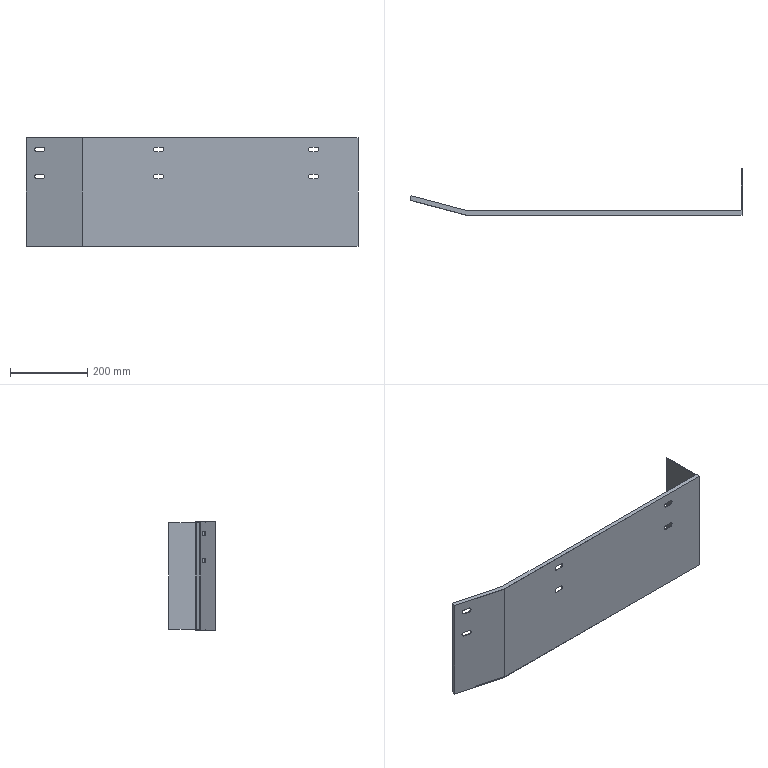Part | SolidWorks | features ICE 3, BossThin 2, LPattern 2, ExtruThin 1 | 1 solid | 48 faces | box 856.99 x 120 x 280 mm | volume 584120 mm3 | plane 30 | cylinder 18 | commonest cylinder face diameters 12 x18
STEP:
#1=CARTESIAN_POINT('',(-808.631,27.69,178.));
#2=VERTEX_POINT('',#1);
#3=CARTESIAN_POINT('',(-814.43,29.228,184.));
#4=VERTEX_POINT('',#3);
#5=CARTESIAN_POINT('',(-814.43,29.228,178.));
#6=DIRECTION('',(-0.2563,-0.9666,0.));
#7=DIRECTION('',(0.9666,-0.2563,0.));
#8=AXIS2_PLACEMENT_3D('',#5,#6,#7);
#9=CIRCLE('',#8,6.);
#10=EDGE_CURVE('',#2,#4,#9,.T.);
#11=ORIENTED_EDGE('',*,*,#10,.F.);
#12=CARTESIAN_POINT('',(-809.143,25.757,178.));
#13=VERTEX_POINT('',#12);
#14=CARTESIAN_POINT('',(-808.631,27.69,178.));
#15=DIRECTION('',(-0.2563,-0.9666,0.));
#16=VECTOR('',#15,1000.);
#17=LINE('',#14,#16);
#18=EDGE_CURVE('',#2,#13,#17,.T.);
#19=ORIENTED_EDGE('',*,*,#18,.T.);
#20=CARTESIAN_POINT('',(-814.943,27.295,184.));
#21=VERTEX_POINT('',#20);
#22=CARTESIAN_POINT('',(-814.943,27.295,178.));
#23=DIRECTION('',(-0.2563,-0.9666,0.));
#24=DIRECTION('',(0.9666,-0.2563,0.));
#25=AXIS2_PLACEMENT_3D('',#22,#23,#24);
#26=CIRCLE('',#25,6.);
#27=EDGE_CURVE('',#13,#21,#26,.T.);
#28=ORIENTED_EDGE('',*,*,#27,.T.);
#29=CARTESIAN_POINT('',(-814.43,29.228,184.));
#30=DIRECTION('',(-0.2563,-0.9666,0.));
#31=VECTOR('',#30,1000.);
#32=LINE('',#29,#31);
#33=EDGE_CURVE('',#4,#21,#32,.T.);
#34=ORIENTED_EDGE('',*,*,#33,.F.);
#35=EDGE_LOOP('',(#11,#19,#28,#34));
#36=FACE_OUTER_BOUND('',#35,.T.);
#37=CARTESIAN_POINT('',(-814.43,29.228,178.));
#38=DIRECTION('',(-0.2563,-0.9666,0.));
#39=DIRECTION('',(0.9666,-0.2563,0.));
#40=AXIS2_PLACEMENT_3D('',#37,#38,#39);
#41=CYLINDRICAL_SURFACE('',#40,6.);
#42=ADVANCED_FACE('',(#36),#41,.F.);
#43=CARTESIAN_POINT('',(-808.631,27.69,248.));
#44=VERTEX_POINT('',#43);
#45=CARTESIAN_POINT('',(-814.43,29.228,254.));
#46=VERTEX_POINT('',#45);
#47=CARTESIAN_POINT('',(-814.43,29.228,248.));
#48=DIRECTION('',(-0.2563,-0.9666,0.));
#49=DIRECTION('',(0.9666,-0.2563,0.));
#50=AXIS2_PLACEMENT_3D('',#47,#48,#49);
#51=CIRCLE('',#50,6.);
#52=EDGE_CURVE('',#44,#46,#51,.T.);
#53=ORIENTED_EDGE('',*,*,#52,.F.);
#54=CARTESIAN_POINT('',(-809.143,25.757,248.));
#55=VERTEX_POINT('',#54);
#56=CARTESIAN_POINT('',(-808.631,27.69,248.));
#57=DIRECTION('',(-0.2563,-0.9666,0.));
#58=VECTOR('',#57,1000.);
#59=LINE('',#56,#58);
#60=EDGE_CURVE('',#44,#55,#59,.T.);
#61=ORIENTED_EDGE('',*,*,#60,.T.);
#62=CARTESIAN_POINT('',(-814.943,27.295,254.));
#63=VERTEX_POINT('',#62);
#64=CARTESIAN_POINT('',(-814.943,27.295,248.));
#65=DIRECTION('',(-0.2563,-0.9666,0.));
#66=DIRECTION('',(0.9666,-0.2563,0.));
#67=AXIS2_PLACEMENT_3D('',#64,#65,#66);
#68=CIRCLE('',#67,6.);
#69=EDGE_CURVE('',#55,#63,#68,.T.);
#70=ORIENTED_EDGE('',*,*,#69,.T.);
#71=CARTESIAN_POINT('',(-814.43,29.228,254.));
#72=DIRECTION('',(-0.2563,-0.9666,0.));
#73=VECTOR('',#72,1000.);
#74=LINE('',#71,#73);
#75=EDGE_CURVE('',#46,#63,#74,.T.);
#76=ORIENTED_EDGE('',*,*,#75,.F.);
#77=EDGE_LOOP('',(#53,#61,#70,#76));
#78=FACE_OUTER_BOUND('',#77,.T.);
#79=CARTESIAN_POINT('',(-814.43,29.228,248.));
#80=DIRECTION('',(-0.2563,-0.9666,0.));
#81=DIRECTION('',(0.9666,-0.2563,0.));
#82=AXIS2_PLACEMENT_3D('',#79,#80,#81);
#83=CYLINDRICAL_SURFACE('',#82,6.);
#84=ADVANCED_FACE('',(#78),#83,.F.);
#85=CARTESIAN_POINT('',(-501.5,2.,178.));
#86=VERTEX_POINT('',#85);
#87=CARTESIAN_POINT('',(-507.5,2.,184.));
#88=VERTEX_POINT('',#87);
#89=CARTESIAN_POINT('',(-507.5,2.,178.));
#90=DIRECTION('',(0.,-1.,0.));
#91=DIRECTION('',(1.,0.,0.));
#92=AXIS2_PLACEMENT_3D('',#89,#90,#91);
#93=CIRCLE('',#92,6.);
#94=EDGE_CURVE('',#86,#88,#93,.T.);
#95=ORIENTED_EDGE('',*,*,#94,.F.);
#96=CARTESIAN_POINT('',(-501.5,0.,178.));
#97=VERTEX_POINT('',#96);
#98=CARTESIAN_POINT('',(-501.5,2.,178.));
#99=DIRECTION('',(0.,-1.,0.));
#100=VECTOR('',#99,1000.);
#101=LINE('',#98,#100);
#102=EDGE_CURVE('',#86,#97,#101,.T.);
#103=ORIENTED_EDGE('',*,*,#102,.T.);
#104=CARTESIAN_POINT('',(-507.5,0.,184.));
#105=VERTEX_POINT('',#104);
#106=CARTESIAN_POINT('',(-507.5,0.,178.));
#107=DIRECTION('',(0.,-1.,0.));
#108=DIRECTION('',(1.,0.,0.));
#109=AXIS2_PLACEMENT_3D('',#106,#107,#108);
#110=CIRCLE('',#109,6.);
#111=EDGE_CURVE('',#97,#105,#110,.T.);
#112=ORIENTED_EDGE('',*,*,#111,.T.);
#113=CARTESIAN_POINT('',(-507.5,2.,184.));
#114=DIRECTION('',(0.,-1.,0.));
#115=VECTOR('',#114,1000.);
#116=LINE('',#113,#115);
#117=EDGE_CURVE('',#88,#105,#116,.T.);
#118=ORIENTED_EDGE('',*,*,#117,.F.);
#119=EDGE_LOOP('',(#95,#103,#112,#118));
#120=FACE_OUTER_BOUND('',#119,.T.);
#121=CARTESIAN_POINT('',(-507.5,2.,178.));
#122=DIRECTION('',(0.,-1.,0.));
#123=DIRECTION('',(1.,0.,0.));
#124=AXIS2_PLACEMENT_3D('',#121,#122,#123);
#125=CYLINDRICAL_SURFACE('',#124,6.);
#126=ADVANCED_FACE('',(#120),#125,.F.);
#127=CARTESIAN_POINT('',(-101.5,2.,178.));
#128=VERTEX_POINT('',#127);
#129=CARTESIAN_POINT('',(-107.5,2.,184.));
#130=VERTEX_POINT('',#129);
#131=CARTESIAN_POINT('',(-107.5,2.,178.));
#132=DIRECTION('',(0.,-1.,0.));
#133=DIRECTION('',(1.,0.,0.));
#134=AXIS2_PLACEMENT_3D('',#131,#132,#133);
#135=CIRCLE('',#134,6.);
#136=EDGE_CURVE('',#128,#130,#135,.T.);
#137=ORIENTED_EDGE('',*,*,#136,.F.);
#138=CARTESIAN_POINT('',(-101.5,0.,178.));
#139=VERTEX_POINT('',#138);
#140=CARTESIAN_POINT('',(-101.5,2.,178.));
#141=DIRECTION('',(0.,-1.,0.));
#142=VECTOR('',#141,1000.);
#143=LINE('',#140,#142);
#144=EDGE_CURVE('',#128,#139,#143,.T.);
#145=ORIENTED_EDGE('',*,*,#144,.T.);
#146=CARTESIAN_POINT('',(-107.5,0.,184.));
#147=VERTEX_POINT('',#146);
#148=CARTESIAN_POINT('',(-107.5,0.,178.));
#149=DIRECTION('',(0.,-1.,0.));
#150=DIRECTION('',(1.,0.,0.));
#151=AXIS2_PLACEMENT_3D('',#148,#149,#150);
#152=CIRCLE('',#151,6.);
#153=EDGE_CURVE('',#139,#147,#152,.T.);
#154=ORIENTED_EDGE('',*,*,#153,.T.);
#155=CARTESIAN_POINT('',(-107.5,2.,184.));
#156=DIRECTION('',(0.,-1.,0.));
#157=VECTOR('',#156,1000.);
#158=LINE('',#155,#157);
#159=EDGE_CURVE('',#130,#147,#158,.T.);
#160=ORIENTED_EDGE('',*,*,#159,.F.);
#161=EDGE_LOOP('',(#137,#145,#154,#160));
#162=FACE_OUTER_BOUND('',#161,.T.);
#163=CARTESIAN_POINT('',(-107.5,2.,178.));
#164=DIRECTION('',(0.,-1.,0.));
#165=DIRECTION('',(1.,0.,0.));
#166=AXIS2_PLACEMENT_3D('',#163,#164,#165);
#167=CYLINDRICAL_SURFACE('',#166,6.);
#168=ADVANCED_FACE('',(#162),#167,.F.);
#169=CARTESIAN_POINT('',(-501.5,2.,248.));
#170=VERTEX_POINT('',#169);
#171=CARTESIAN_POINT('',(-507.5,2.,254.));
#172=VERTEX_POINT('',#171);
#173=CARTESIAN_POINT('',(-507.5,2.,248.));
#174=DIRECTION('',(0.,-1.,0.));
#175=DIRECTION('',(1.,0.,0.));
#176=AXIS2_PLACEMENT_3D('',#173,#174,#175);
#177=CIRCLE('',#176,6.);
#178=EDGE_CURVE('',#170,#172,#177,.T.);
#179=ORIENTED_EDGE('',*,*,#178,.F.);
#180=CARTESIAN_POINT('',(-501.5,0.,248.));
#181=VERTEX_POINT('',#180);
#182=CARTESIAN_POINT('',(-501.5,2.,248.));
#183=DIRECTION('',(0.,-1.,0.));
#184=VECTOR('',#183,1000.);
#185=LINE('',#182,#184);
#186=EDGE_CURVE('',#170,#181,#185,.T.);
#187=ORIENTED_EDGE('',*,*,#186,.T.);
#188=CARTESIAN_POINT('',(-507.5,0.,254.));
#189=VERTEX_POINT('',#188);
#190=CARTESIAN_POINT('',(-507.5,0.,248.));
#191=DIRECTION('',(0.,-1.,0.));
#192=DIRECTION('',(1.,0.,0.));
#193=AXIS2_PLACEMENT_3D('',#190,#191,#192);
#194=CIRCLE('',#193,6.);
#195=EDGE_CURVE('',#181,#189,#194,.T.);
#196=ORIENTED_EDGE('',*,*,#195,.T.);
#197=CARTESIAN_POINT('',(-507.5,2.,254.));
#198=DIRECTION('',(0.,-1.,0.));
#199=VECTOR('',#198,1000.);
#200=LINE('',#197,#199);
#201=EDGE_CURVE('',#172,#189,#200,.T.);
#202=ORIENTED_EDGE('',*,*,#201,.F.);
#203=EDGE_LOOP('',(#179,#187,#196,#202));
#204=FACE_OUTER_BOUND('',#203,.T.);
#205=CARTESIAN_POINT('',(-507.5,2.,248.));
#206=DIRECTION('',(0.,-1.,0.));
#207=DIRECTION('',(1.,0.,0.));
#208=AXIS2_PLACEMENT_3D('',#205,#206,#207);
#209=CYLINDRICAL_SURFACE('',#208,6.);
#210=ADVANCED_FACE('',(#204),#209,.F.);
#211=CARTESIAN_POINT('',(-101.5,2.,248.));
#212=VERTEX_POINT('',#211);
#213=CARTESIAN_POINT('',(-107.5,2.,254.));
#214=VERTEX_POINT('',#213);
#215=CARTESIAN_POINT('',(-107.5,2.,248.));
#216=DIRECTION('',(0.,-1.,0.));
#217=DIRECTION('',(1.,0.,0.));
#218=AXIS2_PLACEMENT_3D('',#215,#216,#217);
#219=CIRCLE('',#218,6.);
#220=EDGE_CURVE('',#212,#214,#219,.T.);
#221=ORIENTED_EDGE('',*,*,#220,.F.);
#222=CARTESIAN_POINT('',(-101.5,0.,248.));
#223=VERTEX_POINT('',#222);
#224=CARTESIAN_POINT('',(-101.5,2.,248.));
#225=DIRECTION('',(0.,-1.,0.));
#226=VECTOR('',#225,1000.);
#227=LINE('',#224,#226);
#228=EDGE_CURVE('',#212,#223,#227,.T.);
#229=ORIENTED_EDGE('',*,*,#228,.T.);
#230=CARTESIAN_POINT('',(-107.5,0.,254.));
#231=VERTEX_POINT('',#230);
#232=CARTESIAN_POINT('',(-107.5,0.,248.));
#233=DIRECTION('',(0.,-1.,0.));
#234=DIRECTION('',(1.,0.,0.));
#235=AXIS2_PLACEMENT_3D('',#232,#233,#234);
#236=CIRCLE('',#235,6.);
#237=EDGE_CURVE('',#223,#231,#236,.T.);
#238=ORIENTED_EDGE('',*,*,#237,.T.);
#239=CARTESIAN_POINT('',(-107.5,2.,254.));
#240=DIRECTION('',(0.,-1.,0.));
#241=VECTOR('',#240,1000.);
#242=LINE('',#239,#241);
#243=EDGE_CURVE('',#214,#231,#242,.T.);
#244=ORIENTED_EDGE('',*,*,#243,.F.);
#245=EDGE_LOOP('',(#221,#229,#238,#244));
#246=FACE_OUTER_BOUND('',#245,.T.);
#247=CARTESIAN_POINT('',(-107.5,2.,248.));
#248=DIRECTION('',(0.,-1.,0.));
#249=DIRECTION('',(1.,0.,0.));
#250=AXIS2_PLACEMENT_3D('',#247,#248,#249);
#251=CYLINDRICAL_SURFACE('',#250,6.);
#252=ADVANCED_FACE('',(#246),#251,.F.);
#253=CARTESIAN_POINT('',(-828.929,33.072,254.));
#254=VERTEX_POINT('',#253);
#255=CARTESIAN_POINT('',(-828.929,33.072,254.));
#256=DIRECTION('',(-0.9666,0.2563,0.));
#257=VECTOR('',#256,1000.);
#258=LINE('',#255,#257);
#259=EDGE_CURVE('',#46,#254,#258,.T.);
#260=ORIENTED_EDGE('',*,*,#259,.T.);
#261=CARTESIAN_POINT('',(-828.929,33.072,242.));
#262=VERTEX_POINT('',#261);
#263=CARTESIAN_POINT('',(-828.929,33.072,248.));
#264=DIRECTION('',(-0.2563,-0.9666,0.));
#265=DIRECTION('',(0.9666,-0.2563,0.));
#266=AXIS2_PLACEMENT_3D('',#263,#264,#265);
#267=CIRCLE('',#266,6.);
#268=EDGE_CURVE('',#254,#262,#267,.T.);
#269=ORIENTED_EDGE('',*,*,#268,.T.);
#270=CARTESIAN_POINT('',(-814.43,29.228,242.));
#271=VERTEX_POINT('',#270);
#272=CARTESIAN_POINT('',(-828.929,33.072,242.));
#273=DIRECTION('',(0.9666,-0.2563,0.));
#274=VECTOR('',#273,1000.);
#275=LINE('',#272,#274);
#276=EDGE_CURVE('',#262,#271,#275,.T.);
#277=ORIENTED_EDGE('',*,*,#276,.T.);
#278=CARTESIAN_POINT('',(-814.43,29.228,248.));
#279=DIRECTION('',(-0.2563,-0.9666,0.));
#280=DIRECTION('',(0.9666,-0.2563,0.));
#281=AXIS2_PLACEMENT_3D('',#278,#279,#280);
#282=CIRCLE('',#281,6.);
#283=EDGE_CURVE('',#271,#44,#282,.T.);
#284=ORIENTED_EDGE('',*,*,#283,.T.);
#285=ORIENTED_EDGE('',*,*,#52,.T.);
#286=EDGE_LOOP('',(#260,#269,#277,#284,#285));
#287=FACE_BOUND('',#286,.T.);
#288=CARTESIAN_POINT('',(-828.929,33.072,184.));
#289=VERTEX_POINT('',#288);
#290=CARTESIAN_POINT('',(-828.929,33.072,184.));
#291=DIRECTION('',(-0.9666,0.2563,0.));
#292=VECTOR('',#291,1000.);
#293=LINE('',#290,#292);
#294=EDGE_CURVE('',#4,#289,#293,.T.);
#295=ORIENTED_EDGE('',*,*,#294,.T.);
#296=CARTESIAN_POINT('',(-828.929,33.072,172.));
#297=VERTEX_POINT('',#296);
#298=CARTESIAN_POINT('',(-828.929,33.072,178.));
#299=DIRECTION('',(-0.2563,-0.9666,0.));
#300=DIRECTION('',(0.9666,-0.2563,0.));
#301=AXIS2_PLACEMENT_3D('',#298,#299,#300);
#302=CIRCLE('',#301,6.);
#303=EDGE_CURVE('',#289,#297,#302,.T.);
#304=ORIENTED_EDGE('',*,*,#303,.T.);
#305=CARTESIAN_POINT('',(-814.43,29.228,172.));
#306=VERTEX_POINT('',#305);
#307=CARTESIAN_POINT('',(-828.929,33.072,172.));
#308=DIRECTION('',(0.9666,-0.2563,0.));
#309=VECTOR('',#308,1000.);
#310=LINE('',#307,#309);
#311=EDGE_CURVE('',#297,#306,#310,.T.);
#312=ORIENTED_EDGE('',*,*,#311,.T.);
#313=CARTESIAN_POINT('',(-814.43,29.228,178.));
#314=DIRECTION('',(-0.2563,-0.9666,0.));
#315=DIRECTION('',(0.9666,-0.2563,0.));
#316=AXIS2_PLACEMENT_3D('',#313,#314,#315);
#317=CIRCLE('',#316,6.);
#318=EDGE_CURVE('',#306,#2,#317,.T.);
#319=ORIENTED_EDGE('',*,*,#318,.T.);
#320=ORIENTED_EDGE('',*,*,#10,.T.);
#321=EDGE_LOOP('',(#295,#304,#312,#319,#320));
#322=FACE_BOUND('',#321,.T.);
#323=CARTESIAN_POINT('',(-854.544,39.864,276.));
#324=VERTEX_POINT('',#323);
#325=CARTESIAN_POINT('',(-854.544,39.864,0.));
#326=VERTEX_POINT('',#325);
#327=CARTESIAN_POINT('',(-854.544,39.864,0.));
#328=DIRECTION('',(0.,0.,-1.));
#329=VECTOR('',#328,1000.);
#330=LINE('',#327,#329);
#331=EDGE_CURVE('',#324,#326,#330,.T.);
#332=ORIENTED_EDGE('',*,*,#331,.F.);
#333=CARTESIAN_POINT('',(-711.739,2.,276.));
#334=VERTEX_POINT('',#333);
#335=CARTESIAN_POINT('',(-711.487,1.933,276.));
#336=DIRECTION('',(-0.9666,0.2563,0.));
#337=VECTOR('',#336,1000.);
#338=LINE('',#335,#337);
#339=EDGE_CURVE('',#334,#324,#338,.T.);
#340=ORIENTED_EDGE('',*,*,#339,.F.);
#341=CARTESIAN_POINT('',(-711.739,2.,0.));
#342=VERTEX_POINT('',#341);
#343=CARTESIAN_POINT('',(-711.739,2.,276.));
#344=DIRECTION('',(0.,0.,-1.));
#345=VECTOR('',#344,1000.);
#346=LINE('',#343,#345);
#347=EDGE_CURVE('',#334,#342,#346,.T.);
#348=ORIENTED_EDGE('',*,*,#347,.T.);
#349=CARTESIAN_POINT('',(-711.487,1.933,0.));
#350=DIRECTION('',(-0.9666,0.2563,0.));
#351=VECTOR('',#350,1000.);
#352=LINE('',#349,#351);
#353=EDGE_CURVE('',#342,#326,#352,.T.);
#354=ORIENTED_EDGE('',*,*,#353,.T.);
#355=EDGE_LOOP('',(#332,#340,#348,#354));
#356=FACE_OUTER_BOUND('',#355,.T.);
#357=CARTESIAN_POINT('',(-711.487,1.933,276.));
#358=DIRECTION('',(-0.2563,-0.9666,0.));
#359=DIRECTION('',(0.9666,-0.2563,0.));
#360=AXIS2_PLACEMENT_3D('',#357,#358,#359);
#361=PLANE('',#360);
#362=ADVANCED_FACE('',(#287,#322,#356),#361,.F.);
#363=ORIENTED_EDGE('',*,*,#339,.T.);
#364=CARTESIAN_POINT('',(-851.981,49.53,276.));
#365=VERTEX_POINT('',#364);
#366=CARTESIAN_POINT('',(-851.981,49.53,276.));
#367=DIRECTION('',(-0.2563,-0.9666,0.));
#368=VECTOR('',#367,1000.);
#369=LINE('',#366,#368);
#370=EDGE_CURVE('',#365,#324,#369,.T.);
#371=ORIENTED_EDGE('',*,*,#370,.F.);
#372=CARTESIAN_POINT('',(-710.436,12.,276.));
#373=VERTEX_POINT('',#372);
#374=CARTESIAN_POINT('',(-708.925,11.599,276.));
#375=DIRECTION('',(-0.9666,0.2563,0.));
#376=VECTOR('',#375,1000.);
#377=LINE('',#374,#376);
#378=EDGE_CURVE('',#373,#365,#377,.T.);
#379=ORIENTED_EDGE('',*,*,#378,.F.);
#380=CARTESIAN_POINT('',(-2.,12.,276.));
#381=VERTEX_POINT('',#380);
#382=CARTESIAN_POINT('',(0.,12.,276.));
#383=DIRECTION('',(-1.,0.,0.));
#384=VECTOR('',#383,1000.);
#385=LINE('',#382,#384);
#386=EDGE_CURVE('',#381,#373,#385,.T.);
#387=ORIENTED_EDGE('',*,*,#386,.F.);
#388=CARTESIAN_POINT('',(-2.,2.,276.));
#389=VERTEX_POINT('',#388);
#390=CARTESIAN_POINT('',(-2.,0.,276.));
#391=DIRECTION('',(0.,-1.,0.));
#392=VECTOR('',#391,1000.);
#393=LINE('',#390,#392);
#394=EDGE_CURVE('',#381,#389,#393,.T.);
#395=ORIENTED_EDGE('',*,*,#394,.T.);
#396=CARTESIAN_POINT('',(0.,2.,276.));
#397=DIRECTION('',(-1.,0.,0.));
#398=VECTOR('',#397,1000.);
#399=LINE('',#396,#398);
#400=EDGE_CURVE('',#389,#334,#399,.T.);
#401=ORIENTED_EDGE('',*,*,#400,.T.);
#402=EDGE_LOOP('',(#363,#371,#379,#387,#395,#401));
#403=FACE_OUTER_BOUND('',#402,.T.);
#404=CARTESIAN_POINT('',(0.,0.,276.));
#405=DIRECTION('',(0.,0.,-1.));
#406=DIRECTION('',(-1.,0.,0.));
#407=AXIS2_PLACEMENT_3D('',#404,#405,#406);
#408=PLANE('',#407);
#409=ADVANCED_FACE('',(#403),#408,.T.);
#410=CARTESIAN_POINT('',(-710.436,12.,0.));
#411=VERTEX_POINT('',#410);
#412=CARTESIAN_POINT('',(-851.981,49.53,0.));
#413=VERTEX_POINT('',#412);
#414=CARTESIAN_POINT('',(-708.925,11.599,0.));
#415=DIRECTION('',(-0.9666,0.2563,0.));
#416=VECTOR('',#415,1000.);
#417=LINE('',#414,#416);
#418=EDGE_CURVE('',#411,#413,#417,.T.);
#419=ORIENTED_EDGE('',*,*,#418,.T.);
#420=CARTESIAN_POINT('',(-851.981,49.53,0.));
#421=DIRECTION('',(-0.2563,-0.9666,0.));
#422=VECTOR('',#421,1000.);
#423=LINE('',#420,#422);
#424=EDGE_CURVE('',#413,#326,#423,.T.);
#425=ORIENTED_EDGE('',*,*,#424,.T.);
#426=ORIENTED_EDGE('',*,*,#353,.F.);
#427=CARTESIAN_POINT('',(-2.,2.,0.));
#428=VERTEX_POINT('',#427);
#429=CARTESIAN_POINT('',(0.,2.,0.));
#430=DIRECTION('',(-1.,0.,0.));
#431=VECTOR('',#430,1000.);
#432=LINE('',#429,#431);
#433=EDGE_CURVE('',#428,#342,#432,.T.);
#434=ORIENTED_EDGE('',*,*,#433,.F.);
#435=CARTESIAN_POINT('',(-2.,12.,0.));
#436=VERTEX_POINT('',#435);
#437=CARTESIAN_POINT('',(-2.,0.,0.));
#438=DIRECTION('',(0.,-1.,0.));
#439=VECTOR('',#438,1000.);
#440=LINE('',#437,#439);
#441=EDGE_CURVE('',#436,#428,#440,.T.);
#442=ORIENTED_EDGE('',*,*,#441,.F.);
#443=CARTESIAN_POINT('',(0.,12.,0.));
#444=DIRECTION('',(-1.,0.,0.));
#445=VECTOR('',#444,1000.);
#446=LINE('',#443,#445);
#447=EDGE_CURVE('',#436,#411,#446,.T.);
#448=ORIENTED_EDGE('',*,*,#447,.T.);
#449=EDGE_LOOP('',(#419,#425,#426,#434,#442,#448));
#450=FACE_OUTER_BOUND('',#449,.T.);
#451=CARTESIAN_POINT('',(0.,0.,0.));
#452=DIRECTION('',(0.,0.,1.));
#453=DIRECTION('',(1.,0.,0.));
#454=AXIS2_PLACEMENT_3D('',#451,#452,#453);
#455=PLANE('',#454);
#456=ADVANCED_FACE('',(#450),#455,.T.);
#457=CARTESIAN_POINT('',(0.,120.,0.));
#458=VERTEX_POINT('',#457);
#459=CARTESIAN_POINT('',(0.,12.,0.));
#460=VERTEX_POINT('',#459);
#461=CARTESIAN_POINT('',(0.,0.,0.));
#462=DIRECTION('',(0.,-1.,0.));
#463=VECTOR('',#462,1000.);
#464=LINE('',#461,#463);
#465=EDGE_CURVE('',#458,#460,#464,.T.);
#466=ORIENTED_EDGE('',*,*,#465,.T.);
#467=CARTESIAN_POINT('',(0.,12.,0.));
#468=DIRECTION('',(-1.,0.,0.));
#469=VECTOR('',#468,1000.);
#470=LINE('',#467,#469);
#471=EDGE_CURVE('',#460,#436,#470,.T.);
#472=ORIENTED_EDGE('',*,*,#471,.T.);
#473=CARTESIAN_POINT('',(-2.,120.,0.));
#474=VERTEX_POINT('',#473);
#475=CARTESIAN_POINT('',(-2.,0.,0.));
#476=DIRECTION('',(0.,-1.,0.));
#477=VECTOR('',#476,1000.);
#478=LINE('',#475,#477);
#479=EDGE_CURVE('',#474,#436,#478,.T.);
#480=ORIENTED_EDGE('',*,*,#479,.F.);
#481=CARTESIAN_POINT('',(-2.,120.,0.));
#482=DIRECTION('',(1.,0.,0.));
#483=VECTOR('',#482,1000.);
#484=LINE('',#481,#483);
#485=EDGE_CURVE('',#474,#458,#484,.T.);
#486=ORIENTED_EDGE('',*,*,#485,.T.);
#487=EDGE_LOOP('',(#466,#472,#480,#486));
#488=FACE_OUTER_BOUND('',#487,.T.);
#489=CARTESIAN_POINT('',(0.,0.,0.));
#490=DIRECTION('',(0.,0.,-1.));
#491=DIRECTION('',(-1.,0.,0.));
#492=AXIS2_PLACEMENT_3D('',#489,#490,#491);
#493=PLANE('',#492);
#494=ADVANCED_FACE('',(#488),#493,.T.);
#495=CARTESIAN_POINT('',(0.,12.,276.));
#496=VERTEX_POINT('',#495);
#497=CARTESIAN_POINT('',(0.,12.,276.));
#498=DIRECTION('',(-1.,0.,0.));
#499=VECTOR('',#498,1000.);
#500=LINE('',#497,#499);
#501=EDGE_CURVE('',#496,#381,#500,.T.);
#502=ORIENTED_EDGE('',*,*,#501,.F.);
#503=CARTESIAN_POINT('',(0.,120.,276.));
#504=VERTEX_POINT('',#503);
#505=CARTESIAN_POINT('',(0.,0.,276.));
#506=DIRECTION('',(0.,-1.,0.));
#507=VECTOR('',#506,1000.);
#508=LINE('',#505,#507);
#509=EDGE_CURVE('',#504,#496,#508,.T.);
#510=ORIENTED_EDGE('',*,*,#509,.F.);
#511=CARTESIAN_POINT('',(-2.,120.,276.));
#512=VERTEX_POINT('',#511);
#513=CARTESIAN_POINT('',(-2.,120.,276.));
#514=DIRECTION('',(1.,0.,0.));
#515=VECTOR('',#514,1000.);
#516=LINE('',#513,#515);
#517=EDGE_CURVE('',#512,#504,#516,.T.);
#518=ORIENTED_EDGE('',*,*,#517,.F.);
#519=CARTESIAN_POINT('',(-2.,0.,276.));
#520=DIRECTION('',(0.,-1.,0.));
#521=VECTOR('',#520,1000.);
#522=LINE('',#519,#521);
#523=EDGE_CURVE('',#512,#381,#522,.T.);
#524=ORIENTED_EDGE('',*,*,#523,.T.);
#525=EDGE_LOOP('',(#502,#510,#518,#524));
#526=FACE_OUTER_BOUND('',#525,.T.);
#527=CARTESIAN_POINT('',(0.,0.,276.));
#528=DIRECTION('',(0.,0.,-1.));
#529=DIRECTION('',(-1.,0.,0.));
#530=AXIS2_PLACEMENT_3D('',#527,#528,#529);
#531=PLANE('',#530);
#532=ADVANCED_FACE('',(#526),#531,.F.);
#533=CARTESIAN_POINT('',(-853.915,50.043,278.));
#534=VERTEX_POINT('',#533);
#535=CARTESIAN_POINT('',(-853.915,50.043,-2.));
#536=VERTEX_POINT('',#535);
#537=CARTESIAN_POINT('',(-853.915,50.043,278.));
#538=DIRECTION('',(0.,0.,-1.));
#539=VECTOR('',#538,1000.);
#540=LINE('',#537,#539);
#541=EDGE_CURVE('',#534,#536,#540,.T.);
#542=ORIENTED_EDGE('',*,*,#541,.T.);
#543=CARTESIAN_POINT('',(-856.99,38.443,-2.));
#544=VERTEX_POINT('',#543);
#545=CARTESIAN_POINT('',(-853.915,50.043,-2.));
#546=DIRECTION('',(-0.2563,-0.9666,0.));
#547=VECTOR('',#546,1000.);
#548=LINE('',#545,#547);
#549=EDGE_CURVE('',#536,#544,#548,.T.);
#550=ORIENTED_EDGE('',*,*,#549,.T.);
#551=CARTESIAN_POINT('',(-856.99,38.443,278.));
#552=VERTEX_POINT('',#551);
#553=CARTESIAN_POINT('',(-856.99,38.443,276.));
#554=DIRECTION('',(0.,0.,-1.));
#555=VECTOR('',#554,1000.);
#556=LINE('',#553,#555);
#557=EDGE_CURVE('',#552,#544,#556,.T.);
#558=ORIENTED_EDGE('',*,*,#557,.F.);
#559=CARTESIAN_POINT('',(-856.99,38.443,278.));
#560=DIRECTION('',(0.2563,0.9666,0.));
#561=VECTOR('',#560,1000.);
#562=LINE('',#559,#561);
#563=EDGE_CURVE('',#552,#534,#562,.T.);
#564=ORIENTED_EDGE('',*,*,#563,.T.);
#565=EDGE_LOOP('',(#542,#550,#558,#564));
#566=FACE_OUTER_BOUND('',#565,.T.);
#567=CARTESIAN_POINT('',(-856.99,38.443,276.));
#568=DIRECTION('',(-0.9666,0.2563,0.));
#569=DIRECTION('',(-0.2563,-0.9666,0.));
#570=AXIS2_PLACEMENT_3D('',#567,#568,#569);
#571=PLANE('',#570);
#572=ADVANCED_FACE('',(#566),#571,.T.);
#573=CARTESIAN_POINT('',(-829.442,31.139,184.));
#574=VERTEX_POINT('',#573);
#575=CARTESIAN_POINT('',(-829.442,31.139,172.));
#576=VERTEX_POINT('',#575);
#577=CARTESIAN_POINT('',(-829.442,31.139,178.));
#578=DIRECTION('',(-0.2563,-0.9666,0.));
#579=DIRECTION('',(0.9666,-0.2563,0.));
#580=AXIS2_PLACEMENT_3D('',#577,#578,#579);
#581=CIRCLE('',#580,6.);
#582=EDGE_CURVE('',#574,#576,#581,.T.);
#583=ORIENTED_EDGE('',*,*,#582,.F.);
#584=CARTESIAN_POINT('',(-829.442,31.139,184.));
#585=DIRECTION('',(-0.9666,0.2563,0.));
#586=VECTOR('',#585,1000.);
#587=LINE('',#584,#586);
#588=EDGE_CURVE('',#21,#574,#587,.T.);
#589=ORIENTED_EDGE('',*,*,#588,.F.);
#590=ORIENTED_EDGE('',*,*,#27,.F.);
#591=CARTESIAN_POINT('',(-814.943,27.295,172.));
#592=VERTEX_POINT('',#591);
#593=CARTESIAN_POINT('',(-814.943,27.295,178.));
#594=DIRECTION('',(-0.2563,-0.9666,0.));
#595=DIRECTION('',(0.9666,-0.2563,0.));
#596=AXIS2_PLACEMENT_3D('',#593,#594,#595);
#597=CIRCLE('',#596,6.);
#598=EDGE_CURVE('',#592,#13,#597,.T.);
#599=ORIENTED_EDGE('',*,*,#598,.F.);
#600=CARTESIAN_POINT('',(-829.442,31.139,172.));
#601=DIRECTION('',(0.9666,-0.2563,0.));
#602=VECTOR('',#601,1000.);
#603=LINE('',#600,#602);
#604=EDGE_CURVE('',#576,#592,#603,.T.);
#605=ORIENTED_EDGE('',*,*,#604,.F.);
#606=EDGE_LOOP('',(#583,#589,#590,#599,#605));
#607=FACE_BOUND('',#606,.T.);
#608=CARTESIAN_POINT('',(-829.442,31.139,254.));
#609=VERTEX_POINT('',#608);
#610=CARTESIAN_POINT('',(-829.442,31.139,242.));
#611=VERTEX_POINT('',#610);
#612=CARTESIAN_POINT('',(-829.442,31.139,248.));
#613=DIRECTION('',(-0.2563,-0.9666,0.));
#614=DIRECTION('',(0.9666,-0.2563,0.));
#615=AXIS2_PLACEMENT_3D('',#612,#613,#614);
#616=CIRCLE('',#615,6.);
#617=EDGE_CURVE('',#609,#611,#616,.T.);
#618=ORIENTED_EDGE('',*,*,#617,.F.);
#619=CARTESIAN_POINT('',(-829.442,31.139,254.));
#620=DIRECTION('',(-0.9666,0.2563,0.));
#621=VECTOR('',#620,1000.);
#622=LINE('',#619,#621);
#623=EDGE_CURVE('',#63,#609,#622,.T.);
#624=ORIENTED_EDGE('',*,*,#623,.F.);
#625=ORIENTED_EDGE('',*,*,#69,.F.);
#626=CARTESIAN_POINT('',(-814.943,27.295,242.));
#627=VERTEX_POINT('',#626);
#628=CARTESIAN_POINT('',(-814.943,27.295,248.));
#629=DIRECTION('',(-0.2563,-0.9666,0.));
#630=DIRECTION('',(0.9666,-0.2563,0.));
#631=AXIS2_PLACEMENT_3D('',#628,#629,#630);
#632=CIRCLE('',#631,6.);
#633=EDGE_CURVE('',#627,#55,#632,.T.);
#634=ORIENTED_EDGE('',*,*,#633,.F.);
#635=CARTESIAN_POINT('',(-829.442,31.139,242.));
#636=DIRECTION('',(0.9666,-0.2563,0.));
#637=VECTOR('',#636,1000.);
#638=LINE('',#635,#637);
#639=EDGE_CURVE('',#611,#627,#638,.T.);
#640=ORIENTED_EDGE('',*,*,#639,.F.);
#641=EDGE_LOOP('',(#618,#624,#625,#634,#640));
#642=FACE_BOUND('',#641,.T.);
#643=ORIENTED_EDGE('',*,*,#557,.T.);
#644=CARTESIAN_POINT('',(-712.,0.,-2.));
#645=VERTEX_POINT('',#644);
#646=CARTESIAN_POINT('',(-712.,0.,-2.));
#647=DIRECTION('',(-0.9666,0.2563,0.));
#648=VECTOR('',#647,1000.);
#649=LINE('',#646,#648);
#650=EDGE_CURVE('',#645,#544,#649,.T.);
#651=ORIENTED_EDGE('',*,*,#650,.F.);
#652=CARTESIAN_POINT('',(-712.,0.,278.));
#653=VERTEX_POINT('',#652);
#654=CARTESIAN_POINT('',(-712.,0.,276.));
#655=DIRECTION('',(0.,0.,-1.));
#656=VECTOR('',#655,1000.);
#657=LINE('',#654,#656);
#658=EDGE_CURVE('',#653,#645,#657,.T.);
#659=ORIENTED_EDGE('',*,*,#658,.F.);
#660=CARTESIAN_POINT('',(-712.,0.,278.));
#661=DIRECTION('',(-0.9666,0.2563,0.));
#662=VECTOR('',#661,1000.);
#663=LINE('',#660,#662);
#664=EDGE_CURVE('',#653,#552,#663,.T.);
#665=ORIENTED_EDGE('',*,*,#664,.T.);
#666=EDGE_LOOP('',(#643,#651,#659,#665));
#667=FACE_OUTER_BOUND('',#666,.T.);
#668=CARTESIAN_POINT('',(-712.,0.,276.));
#669=DIRECTION('',(-0.2563,-0.9666,0.));
#670=DIRECTION('',(0.9666,-0.2563,0.));
#671=AXIS2_PLACEMENT_3D('',#668,#669,#670);
#672=PLANE('',#671);
#673=ADVANCED_FACE('',(#607,#642,#667),#672,.T.);
#674=CARTESIAN_POINT('',(-522.5,0.,254.));
#675=VERTEX_POINT('',#674);
#676=CARTESIAN_POINT('',(-522.5,0.,242.));
#677=VERTEX_POINT('',#676);
#678=CARTESIAN_POINT('',(-522.5,0.,248.));
#679=DIRECTION('',(0.,-1.,0.));
#680=DIRECTION('',(1.,0.,0.));
#681=AXIS2_PLACEMENT_3D('',#678,#679,#680);
#682=CIRCLE('',#681,6.);
#683=EDGE_CURVE('',#675,#677,#682,.T.);
#684=ORIENTED_EDGE('',*,*,#683,.F.);
#685=CARTESIAN_POINT('',(-522.5,0.,254.));
#686=DIRECTION('',(-1.,0.,0.));
#687=VECTOR('',#686,1000.);
#688=LINE('',#685,#687);
#689=EDGE_CURVE('',#189,#675,#688,.T.);
#690=ORIENTED_EDGE('',*,*,#689,.F.);
#691=ORIENTED_EDGE('',*,*,#195,.F.);
#692=CARTESIAN_POINT('',(-507.5,0.,242.));
#693=VERTEX_POINT('',#692);
#694=CARTESIAN_POINT('',(-507.5,0.,248.));
#695=DIRECTION('',(0.,-1.,0.));
#696=DIRECTION('',(1.,0.,0.));
#697=AXIS2_PLACEMENT_3D('',#694,#695,#696);
#698=CIRCLE('',#697,6.);
#699=EDGE_CURVE('',#693,#181,#698,.T.);
#700=ORIENTED_EDGE('',*,*,#699,.F.);
#701=CARTESIAN_POINT('',(-522.5,0.,242.));
#702=DIRECTION('',(1.,0.,0.));
#703=VECTOR('',#702,1000.);
#704=LINE('',#701,#703);
#705=EDGE_CURVE('',#677,#693,#704,.T.);
#706=ORIENTED_EDGE('',*,*,#705,.F.);
#707=EDGE_LOOP('',(#684,#690,#691,#700,#706));
#708=FACE_BOUND('',#707,.T.);
#709=CARTESIAN_POINT('',(-122.5,0.,254.));
#710=VERTEX_POINT('',#709);
#711=CARTESIAN_POINT('',(-122.5,0.,242.));
#712=VERTEX_POINT('',#711);
#713=CARTESIAN_POINT('',(-122.5,0.,248.));
#714=DIRECTION('',(0.,-1.,0.));
#715=DIRECTION('',(1.,0.,0.));
#716=AXIS2_PLACEMENT_3D('',#713,#714,#715);
#717=CIRCLE('',#716,6.);
#718=EDGE_CURVE('',#710,#712,#717,.T.);
#719=ORIENTED_EDGE('',*,*,#718,.F.);
#720=CARTESIAN_POINT('',(-122.5,0.,254.));
#721=DIRECTION('',(-1.,0.,0.));
#722=VECTOR('',#721,1000.);
#723=LINE('',#720,#722);
#724=EDGE_CURVE('',#231,#710,#723,.T.);
#725=ORIENTED_EDGE('',*,*,#724,.F.);
#726=ORIENTED_EDGE('',*,*,#237,.F.);
#727=CARTESIAN_POINT('',(-107.5,0.,242.));
#728=VERTEX_POINT('',#727);
#729=CARTESIAN_POINT('',(-107.5,0.,248.));
#730=DIRECTION('',(0.,-1.,0.));
#731=DIRECTION('',(1.,0.,0.));
#732=AXIS2_PLACEMENT_3D('',#729,#730,#731);
#733=CIRCLE('',#732,6.);
#734=EDGE_CURVE('',#728,#223,#733,.T.);
#735=ORIENTED_EDGE('',*,*,#734,.F.);
#736=CARTESIAN_POINT('',(-122.5,0.,242.));
#737=DIRECTION('',(1.,0.,0.));
#738=VECTOR('',#737,1000.);
#739=LINE('',#736,#738);
#740=EDGE_CURVE('',#712,#728,#739,.T.);
#741=ORIENTED_EDGE('',*,*,#740,.F.);
#742=EDGE_LOOP('',(#719,#725,#726,#735,#741));
#743=FACE_BOUND('',#742,.T.);
#744=ORIENTED_EDGE('',*,*,#658,.T.);
#745=CARTESIAN_POINT('',(0.,0.,-2.));
#746=VERTEX_POINT('',#745);
#747=CARTESIAN_POINT('',(0.,0.,-2.));
#748=DIRECTION('',(-1.,0.,0.));
#749=VECTOR('',#748,1000.);
#750=LINE('',#747,#749);
#751=EDGE_CURVE('',#746,#645,#750,.T.);
#752=ORIENTED_EDGE('',*,*,#751,.F.);
#753=CARTESIAN_POINT('',(0.,0.,278.));
#754=VERTEX_POINT('',#753);
#755=CARTESIAN_POINT('',(0.,0.,276.));
#756=DIRECTION('',(0.,0.,-1.));
#757=VECTOR('',#756,1000.);
#758=LINE('',#755,#757);
#759=EDGE_CURVE('',#754,#746,#758,.T.);
#760=ORIENTED_EDGE('',*,*,#759,.F.);
#761=CARTESIAN_POINT('',(0.,0.,278.));
#762=DIRECTION('',(-1.,0.,0.));
#763=VECTOR('',#762,1000.);
#764=LINE('',#761,#763);
#765=EDGE_CURVE('',#754,#653,#764,.T.);
#766=ORIENTED_EDGE('',*,*,#765,.T.);
#767=EDGE_LOOP('',(#744,#752,#760,#766));
#768=FACE_OUTER_BOUND('',#767,.T.);
#769=CARTESIAN_POINT('',(-122.5,0.,184.));
#770=VERTEX_POINT('',#769);
#771=CARTESIAN_POINT('',(-122.5,0.,172.));
#772=VERTEX_POINT('',#771);
#773=CARTESIAN_POINT('',(-122.5,0.,178.));
#774=DIRECTION('',(0.,-1.,0.));
#775=DIRECTION('',(1.,0.,0.));
#776=AXIS2_PLACEMENT_3D('',#773,#774,#775);
#777=CIRCLE('',#776,6.);
#778=EDGE_CURVE('',#770,#772,#777,.T.);
#779=ORIENTED_EDGE('',*,*,#778,.F.);
#780=CARTESIAN_POINT('',(-122.5,0.,184.));
#781=DIRECTION('',(-1.,0.,0.));
#782=VECTOR('',#781,1000.);
#783=LINE('',#780,#782);
#784=EDGE_CURVE('',#147,#770,#783,.T.);
#785=ORIENTED_EDGE('',*,*,#784,.F.);
#786=ORIENTED_EDGE('',*,*,#153,.F.);
#787=CARTESIAN_POINT('',(-107.5,0.,172.));
#788=VERTEX_POINT('',#787);
#789=CARTESIAN_POINT('',(-107.5,0.,178.));
#790=DIRECTION('',(0.,-1.,0.));
#791=DIRECTION('',(1.,0.,0.));
#792=AXIS2_PLACEMENT_3D('',#789,#790,#791);
#793=CIRCLE('',#792,6.);
#794=EDGE_CURVE('',#788,#139,#793,.T.);
#795=ORIENTED_EDGE('',*,*,#794,.F.);
#796=CARTESIAN_POINT('',(-122.5,0.,172.));
#797=DIRECTION('',(1.,0.,0.));
#798=VECTOR('',#797,1000.);
#799=LINE('',#796,#798);
#800=EDGE_CURVE('',#772,#788,#799,.T.);
#801=ORIENTED_EDGE('',*,*,#800,.F.);
#802=EDGE_LOOP('',(#779,#785,#786,#795,#801));
#803=FACE_BOUND('',#802,.T.);
#804=CARTESIAN_POINT('',(-522.5,0.,184.));
#805=VERTEX_POINT('',#804);
#806=CARTESIAN_POINT('',(-522.5,0.,172.));
#807=VERTEX_POINT('',#806);
#808=CARTESIAN_POINT('',(-522.5,0.,178.));
#809=DIRECTION('',(0.,-1.,0.));
#810=DIRECTION('',(1.,0.,0.));
#811=AXIS2_PLACEMENT_3D('',#808,#809,#810);
#812=CIRCLE('',#811,6.);
#813=EDGE_CURVE('',#805,#807,#812,.T.);
#814=ORIENTED_EDGE('',*,*,#813,.F.);
#815=CARTESIAN_POINT('',(-522.5,0.,184.));
#816=DIRECTION('',(-1.,0.,0.));
#817=VECTOR('',#816,1000.);
#818=LINE('',#815,#817);
#819=EDGE_CURVE('',#105,#805,#818,.T.);
#820=ORIENTED_EDGE('',*,*,#819,.F.);
#821=ORIENTED_EDGE('',*,*,#111,.F.);
#822=CARTESIAN_POINT('',(-507.5,0.,172.));
#823=VERTEX_POINT('',#822);
#824=CARTESIAN_POINT('',(-507.5,0.,178.));
#825=DIRECTION('',(0.,-1.,0.));
#826=DIRECTION('',(1.,0.,0.));
#827=AXIS2_PLACEMENT_3D('',#824,#825,#826);
#828=CIRCLE('',#827,6.);
#829=EDGE_CURVE('',#823,#97,#828,.T.);
#830=ORIENTED_EDGE('',*,*,#829,.F.);
#831=CARTESIAN_POINT('',(-522.5,0.,172.));
#832=DIRECTION('',(1.,0.,0.));
#833=VECTOR('',#832,1000.);
#834=LINE('',#831,#833);
#835=EDGE_CURVE('',#807,#823,#834,.T.);
#836=ORIENTED_EDGE('',*,*,#835,.F.);
#837=EDGE_LOOP('',(#814,#820,#821,#830,#836));
#838=FACE_BOUND('',#837,.T.);
#839=CARTESIAN_POINT('',(0.,0.,276.));
#840=DIRECTION('',(0.,-1.,0.));
#841=DIRECTION('',(1.,0.,0.));
#842=AXIS2_PLACEMENT_3D('',#839,#840,#841);
#843=PLANE('',#842);
#844=ADVANCED_FACE('',(#708,#743,#768,#803,#838),#843,.T.);
#845=ORIENTED_EDGE('',*,*,#465,.F.);
#846=CARTESIAN_POINT('',(0.,120.,276.));
#847=DIRECTION('',(0.,0.,-1.));
#848=VECTOR('',#847,1000.);
#849=LINE('',#846,#848);
#850=EDGE_CURVE('',#504,#458,#849,.T.);
#851=ORIENTED_EDGE('',*,*,#850,.F.);
#852=ORIENTED_EDGE('',*,*,#509,.T.);
#853=CARTESIAN_POINT('',(0.,12.,278.));
#854=VERTEX_POINT('',#853);
#855=CARTESIAN_POINT('',(0.,12.,278.));
#856=DIRECTION('',(0.,0.,-1.));
#857=VECTOR('',#856,1000.);
#858=LINE('',#855,#857);
#859=EDGE_CURVE('',#854,#496,#858,.T.);
#860=ORIENTED_EDGE('',*,*,#859,.F.);
#861=CARTESIAN_POINT('',(0.,12.,278.));
#862=DIRECTION('',(0.,-1.,0.));
#863=VECTOR('',#862,1000.);
#864=LINE('',#861,#863);
#865=EDGE_CURVE('',#854,#754,#864,.T.);
#866=ORIENTED_EDGE('',*,*,#865,.T.);
#867=ORIENTED_EDGE('',*,*,#759,.T.);
#868=CARTESIAN_POINT('',(0.,12.,-2.));
#869=VERTEX_POINT('',#868);
#870=CARTESIAN_POINT('',(0.,0.,-2.));
#871=DIRECTION('',(0.,1.,0.));
#872=VECTOR('',#871,1000.);
#873=LINE('',#870,#872);
#874=EDGE_CURVE('',#746,#869,#873,.T.);
#875=ORIENTED_EDGE('',*,*,#874,.T.);
#876=CARTESIAN_POINT('',(0.,12.,-2.));
#877=DIRECTION('',(0.,0.,1.));
#878=VECTOR('',#877,1000.);
#879=LINE('',#876,#878);
#880=EDGE_CURVE('',#869,#460,#879,.T.);
#881=ORIENTED_EDGE('',*,*,#880,.T.);
#882=EDGE_LOOP('',(#845,#851,#852,#860,#866,#867,#875,#881));
#883=FACE_OUTER_BOUND('',#882,.T.);
#884=CARTESIAN_POINT('',(0.,0.,276.));
#885=DIRECTION('',(1.,0.,0.));
#886=DIRECTION('',(0.,0.,-1.));
#887=AXIS2_PLACEMENT_3D('',#884,#885,#886);
#888=PLANE('',#887);
#889=ADVANCED_FACE('',(#883),#888,.T.);
#890=ORIENTED_EDGE('',*,*,#485,.F.);
#891=CARTESIAN_POINT('',(-2.,120.,276.));
#892=DIRECTION('',(0.,0.,-1.));
#893=VECTOR('',#892,1000.);
#894=LINE('',#891,#893);
#895=EDGE_CURVE('',#512,#474,#894,.T.);
#896=ORIENTED_EDGE('',*,*,#895,.F.);
#897=ORIENTED_EDGE('',*,*,#517,.T.);
#898=ORIENTED_EDGE('',*,*,#850,.T.);
#899=EDGE_LOOP('',(#890,#896,#897,#898));
#900=FACE_OUTER_BOUND('',#899,.T.);
#901=CARTESIAN_POINT('',(-2.,120.,276.));
#902=DIRECTION('',(0.,1.,0.));
#903=DIRECTION('',(0.,0.,1.));
#904=AXIS2_PLACEMENT_3D('',#901,#902,#903);
#905=PLANE('',#904);
#906=ADVANCED_FACE('',(#900),#905,.T.);
#907=ORIENTED_EDGE('',*,*,#479,.T.);
#908=ORIENTED_EDGE('',*,*,#441,.T.);
#909=CARTESIAN_POINT('',(-2.,2.,276.));
#910=DIRECTION('',(0.,0.,-1.));
#911=VECTOR('',#910,1000.);
#912=LINE('',#909,#911);
#913=EDGE_CURVE('',#389,#428,#912,.T.);
#914=ORIENTED_EDGE('',*,*,#913,.F.);
#915=ORIENTED_EDGE('',*,*,#394,.F.);
#916=ORIENTED_EDGE('',*,*,#523,.F.);
#917=ORIENTED_EDGE('',*,*,#895,.T.);
#918=EDGE_LOOP('',(#907,#908,#914,#915,#916,#917));
#919=FACE_OUTER_BOUND('',#918,.T.);
#920=CARTESIAN_POINT('',(-2.,0.,276.));
#921=DIRECTION('',(1.,0.,0.));
#922=DIRECTION('',(0.,0.,-1.));
#923=AXIS2_PLACEMENT_3D('',#920,#921,#922);
#924=PLANE('',#923);
#925=ADVANCED_FACE('',(#919),#924,.F.);
#926=CARTESIAN_POINT('',(-522.5,2.,254.));
#927=VERTEX_POINT('',#926);
#928=CARTESIAN_POINT('',(-522.5,2.,254.));
#929=DIRECTION('',(-1.,0.,0.));
#930=VECTOR('',#929,1000.);
#931=LINE('',#928,#930);
#932=EDGE_CURVE('',#172,#927,#931,.T.);
#933=ORIENTED_EDGE('',*,*,#932,.T.);
#934=CARTESIAN_POINT('',(-522.5,2.,242.));
#935=VERTEX_POINT('',#934);
#936=CARTESIAN_POINT('',(-522.5,2.,248.));
#937=DIRECTION('',(0.,-1.,0.));
#938=DIRECTION('',(1.,0.,0.));
#939=AXIS2_PLACEMENT_3D('',#936,#937,#938);
#940=CIRCLE('',#939,6.);
#941=EDGE_CURVE('',#927,#935,#940,.T.);
#942=ORIENTED_EDGE('',*,*,#941,.T.);
#943=CARTESIAN_POINT('',(-507.5,2.,242.));
#944=VERTEX_POINT('',#943);
#945=CARTESIAN_POINT('',(-522.5,2.,242.));
#946=DIRECTION('',(1.,0.,0.));
#947=VECTOR('',#946,1000.);
#948=LINE('',#945,#947);
#949=EDGE_CURVE('',#935,#944,#948,.T.);
#950=ORIENTED_EDGE('',*,*,#949,.T.);
#951=CARTESIAN_POINT('',(-507.5,2.,248.));
#952=DIRECTION('',(0.,-1.,0.));
#953=DIRECTION('',(1.,0.,0.));
#954=AXIS2_PLACEMENT_3D('',#951,#952,#953);
#955=CIRCLE('',#954,6.);
#956=EDGE_CURVE('',#944,#170,#955,.T.);
#957=ORIENTED_EDGE('',*,*,#956,.T.);
#958=ORIENTED_EDGE('',*,*,#178,.T.);
#959=EDGE_LOOP('',(#933,#942,#950,#957,#958));
#960=FACE_BOUND('',#959,.T.);
#961=CARTESIAN_POINT('',(-122.5,2.,254.));
#962=VERTEX_POINT('',#961);
#963=CARTESIAN_POINT('',(-122.5,2.,254.));
#964=DIRECTION('',(-1.,0.,0.));
#965=VECTOR('',#964,1000.);
#966=LINE('',#963,#965);
#967=EDGE_CURVE('',#214,#962,#966,.T.);
#968=ORIENTED_EDGE('',*,*,#967,.T.);
#969=CARTESIAN_POINT('',(-122.5,2.,242.));
#970=VERTEX_POINT('',#969);
#971=CARTESIAN_POINT('',(-122.5,2.,248.));
#972=DIRECTION('',(0.,-1.,0.));
#973=DIRECTION('',(1.,0.,0.));
#974=AXIS2_PLACEMENT_3D('',#971,#972,#973);
#975=CIRCLE('',#974,6.);
#976=EDGE_CURVE('',#962,#970,#975,.T.);
#977=ORIENTED_EDGE('',*,*,#976,.T.);
#978=CARTESIAN_POINT('',(-107.5,2.,242.));
#979=VERTEX_POINT('',#978);
#980=CARTESIAN_POINT('',(-122.5,2.,242.));
#981=DIRECTION('',(1.,0.,0.));
#982=VECTOR('',#981,1000.);
#983=LINE('',#980,#982);
#984=EDGE_CURVE('',#970,#979,#983,.T.);
#985=ORIENTED_EDGE('',*,*,#984,.T.);
#986=CARTESIAN_POINT('',(-107.5,2.,248.));
#987=DIRECTION('',(0.,-1.,0.));
#988=DIRECTION('',(1.,0.,0.));
#989=AXIS2_PLACEMENT_3D('',#986,#987,#988);
#990=CIRCLE('',#989,6.);
#991=EDGE_CURVE('',#979,#212,#990,.T.);
#992=ORIENTED_EDGE('',*,*,#991,.T.);
#993=ORIENTED_EDGE('',*,*,#220,.T.);
#994=EDGE_LOOP('',(#968,#977,#985,#992,#993));
#995=FACE_BOUND('',#994,.T.);
#996=ORIENTED_EDGE('',*,*,#433,.T.);
#997=ORIENTED_EDGE('',*,*,#347,.F.);
#998=ORIENTED_EDGE('',*,*,#400,.F.);
#999=ORIENTED_EDGE('',*,*,#913,.T.);
#1000=EDGE_LOOP('',(#996,#997,#998,#999));
#1001=FACE_OUTER_BOUND('',#1000,.T.);
#1002=CARTESIAN_POINT('',(-122.5,2.,184.));
#1003=VERTEX_POINT('',#1002);
#1004=CARTESIAN_POINT('',(-122.5,2.,172.));
#1005=VERTEX_POINT('',#1004);
#1006=CARTESIAN_POINT('',(-122.5,2.,178.));
#1007=DIRECTION('',(0.,-1.,0.));
#1008=DIRECTION('',(1.,0.,0.));
#1009=AXIS2_PLACEMENT_3D('',#1006,#1007,#1008);
#1010=CIRCLE('',#1009,6.);
#1011=EDGE_CURVE('',#1003,#1005,#1010,.T.);
#1012=ORIENTED_EDGE('',*,*,#1011,.T.);
#1013=CARTESIAN_POINT('',(-107.5,2.,172.));
#1014=VERTEX_POINT('',#1013);
#1015=CARTESIAN_POINT('',(-122.5,2.,172.));
#1016=DIRECTION('',(1.,0.,0.));
#1017=VECTOR('',#1016,1000.);
#1018=LINE('',#1015,#1017);
#1019=EDGE_CURVE('',#1005,#1014,#1018,.T.);
#1020=ORIENTED_EDGE('',*,*,#1019,.T.);
#1021=CARTESIAN_POINT('',(-107.5,2.,178.));
#1022=DIRECTION('',(0.,-1.,0.));
#1023=DIRECTION('',(1.,0.,0.));
#1024=AXIS2_PLACEMENT_3D('',#1021,#1022,#1023);
#1025=CIRCLE('',#1024,6.);
#1026=EDGE_CURVE('',#1014,#128,#1025,.T.);
#1027=ORIENTED_EDGE('',*,*,#1026,.T.);
#1028=ORIENTED_EDGE('',*,*,#136,.T.);
#1029=CARTESIAN_POINT('',(-122.5,2.,184.));
#1030=DIRECTION('',(-1.,0.,0.));
#1031=VECTOR('',#1030,1000.);
#1032=LINE('',#1029,#1031);
#1033=EDGE_CURVE('',#130,#1003,#1032,.T.);
#1034=ORIENTED_EDGE('',*,*,#1033,.T.);
#1035=EDGE_LOOP('',(#1012,#1020,#1027,#1028,#1034));
#1036=FACE_BOUND('',#1035,.T.);
#1037=CARTESIAN_POINT('',(-522.5,2.,184.));
#1038=VERTEX_POINT('',#1037);
#1039=CARTESIAN_POINT('',(-522.5,2.,172.));
#1040=VERTEX_POINT('',#1039);
#1041=CARTESIAN_POINT('',(-522.5,2.,178.));
#1042=DIRECTION('',(0.,-1.,0.));
#1043=DIRECTION('',(1.,0.,0.));
#1044=AXIS2_PLACEMENT_3D('',#1041,#1042,#1043);
#1045=CIRCLE('',#1044,6.);
#1046=EDGE_CURVE('',#1038,#1040,#1045,.T.);
#1047=ORIENTED_EDGE('',*,*,#1046,.T.);
#1048=CARTESIAN_POINT('',(-507.5,2.,172.));
#1049=VERTEX_POINT('',#1048);
#1050=CARTESIAN_POINT('',(-522.5,2.,172.));
#1051=DIRECTION('',(1.,0.,0.));
#1052=VECTOR('',#1051,1000.);
#1053=LINE('',#1050,#1052);
#1054=EDGE_CURVE('',#1040,#1049,#1053,.T.);
#1055=ORIENTED_EDGE('',*,*,#1054,.T.);
#1056=CARTESIAN_POINT('',(-507.5,2.,178.));
#1057=DIRECTION('',(0.,-1.,0.));
#1058=DIRECTION('',(1.,0.,0.));
#1059=AXIS2_PLACEMENT_3D('',#1056,#1057,#1058);
#1060=CIRCLE('',#1059,6.);
#1061=EDGE_CURVE('',#1049,#86,#1060,.T.);
#1062=ORIENTED_EDGE('',*,*,#1061,.T.);
#1063=ORIENTED_EDGE('',*,*,#94,.T.);
#1064=CARTESIAN_POINT('',(-522.5,2.,184.));
#1065=DIRECTION('',(-1.,0.,0.));
#1066=VECTOR('',#1065,1000.);
#1067=LINE('',#1064,#1066);
#1068=EDGE_CURVE('',#88,#1038,#1067,.T.);
#1069=ORIENTED_EDGE('',*,*,#1068,.T.);
#1070=EDGE_LOOP('',(#1047,#1055,#1062,#1063,#1069));
#1071=FACE_BOUND('',#1070,.T.);
#1072=CARTESIAN_POINT('',(0.,2.,276.));
#1073=DIRECTION('',(0.,-1.,0.));
#1074=DIRECTION('',(1.,0.,0.));
#1075=AXIS2_PLACEMENT_3D('',#1072,#1073,#1074);
#1076=PLANE('',#1075);
#1077=ADVANCED_FACE('',(#960,#995,#1001,#1036,#1071),#1076,.F.);
#1078=ORIENTED_EDGE('',*,*,#378,.T.);
#1079=CARTESIAN_POINT('',(-851.981,49.53,0.));
#1080=DIRECTION('',(0.,0.,-1.));
#1081=VECTOR('',#1080,1000.);
#1082=LINE('',#1079,#1081);
#1083=EDGE_CURVE('',#365,#413,#1082,.T.);
#1084=ORIENTED_EDGE('',*,*,#1083,.T.);
#1085=ORIENTED_EDGE('',*,*,#418,.F.);
#1086=CARTESIAN_POINT('',(-710.436,12.,-2.));
#1087=VERTEX_POINT('',#1086);
#1088=CARTESIAN_POINT('',(-710.436,12.,-2.));
#1089=DIRECTION('',(0.,0.,1.));
#1090=VECTOR('',#1089,1000.);
#1091=LINE('',#1088,#1090);
#1092=EDGE_CURVE('',#1087,#411,#1091,.T.);
#1093=ORIENTED_EDGE('',*,*,#1092,.F.);
#1094=CARTESIAN_POINT('',(-708.925,11.599,-2.));
#1095=DIRECTION('',(-0.9666,0.2563,0.));
#1096=VECTOR('',#1095,1000.);
#1097=LINE('',#1094,#1096);
#1098=EDGE_CURVE('',#1087,#536,#1097,.T.);
#1099=ORIENTED_EDGE('',*,*,#1098,.T.);
#1100=ORIENTED_EDGE('',*,*,#541,.F.);
#1101=CARTESIAN_POINT('',(-710.436,12.,278.));
#1102=VERTEX_POINT('',#1101);
#1103=CARTESIAN_POINT('',(-708.925,11.599,278.));
#1104=DIRECTION('',(-0.9666,0.2563,0.));
#1105=VECTOR('',#1104,1000.);
#1106=LINE('',#1103,#1105);
#1107=EDGE_CURVE('',#1102,#534,#1106,.T.);
#1108=ORIENTED_EDGE('',*,*,#1107,.F.);
#1109=CARTESIAN_POINT('',(-710.436,12.,278.));
#1110=DIRECTION('',(0.,0.,-1.));
#1111=VECTOR('',#1110,1000.);
#1112=LINE('',#1109,#1111);
#1113=EDGE_CURVE('',#1102,#373,#1112,.T.);
#1114=ORIENTED_EDGE('',*,*,#1113,.T.);
#1115=EDGE_LOOP('',(#1078,#1084,#1085,#1093,#1099,#1100,#1108,#1114));
#1116=FACE_OUTER_BOUND('',#1115,.T.);
#1117=CARTESIAN_POINT('',(-708.925,11.599,278.));
#1118=DIRECTION('',(-0.2563,-0.9666,0.));
#1119=DIRECTION('',(0.9666,-0.2563,0.));
#1120=AXIS2_PLACEMENT_3D('',#1117,#1118,#1119);
#1121=PLANE('',#1120);
#1122=ADVANCED_FACE('',(#1116),#1121,.F.);
#1123=ORIENTED_EDGE('',*,*,#501,.T.);
#1124=ORIENTED_EDGE('',*,*,#386,.T.);
#1125=ORIENTED_EDGE('',*,*,#1113,.F.);
#1126=CARTESIAN_POINT('',(0.,12.,278.));
#1127=DIRECTION('',(-1.,0.,0.));
#1128=VECTOR('',#1127,1000.);
#1129=LINE('',#1126,#1128);
#1130=EDGE_CURVE('',#854,#1102,#1129,.T.);
#1131=ORIENTED_EDGE('',*,*,#1130,.F.);
#1132=ORIENTED_EDGE('',*,*,#859,.T.);
#1133=EDGE_LOOP('',(#1123,#1124,#1125,#1131,#1132));
#1134=FACE_OUTER_BOUND('',#1133,.T.);
#1135=CARTESIAN_POINT('',(0.,12.,278.));
#1136=DIRECTION('',(0.,-1.,0.));
#1137=DIRECTION('',(1.,0.,0.));
#1138=AXIS2_PLACEMENT_3D('',#1135,#1136,#1137);
#1139=PLANE('',#1138);
#1140=ADVANCED_FACE('',(#1134),#1139,.F.);
#1141=ORIENTED_EDGE('',*,*,#1107,.T.);
#1142=ORIENTED_EDGE('',*,*,#563,.F.);
#1143=ORIENTED_EDGE('',*,*,#664,.F.);
#1144=ORIENTED_EDGE('',*,*,#765,.F.);
#1145=ORIENTED_EDGE('',*,*,#865,.F.);
#1146=ORIENTED_EDGE('',*,*,#1130,.T.);
#1147=EDGE_LOOP('',(#1141,#1142,#1143,#1144,#1145,#1146));
#1148=FACE_OUTER_BOUND('',#1147,.T.);
#1149=CARTESIAN_POINT('',(0.,0.,278.));
#1150=DIRECTION('',(0.,0.,-1.));
#1151=DIRECTION('',(-1.,0.,0.));
#1152=AXIS2_PLACEMENT_3D('',#1149,#1150,#1151);
#1153=PLANE('',#1152);
#1154=ADVANCED_FACE('',(#1148),#1153,.F.);
#1155=ORIENTED_EDGE('',*,*,#471,.F.);
#1156=ORIENTED_EDGE('',*,*,#880,.F.);
#1157=CARTESIAN_POINT('',(0.,12.,-2.));
#1158=DIRECTION('',(-1.,0.,0.));
#1159=VECTOR('',#1158,1000.);
#1160=LINE('',#1157,#1159);
#1161=EDGE_CURVE('',#869,#1087,#1160,.T.);
#1162=ORIENTED_EDGE('',*,*,#1161,.T.);
#1163=ORIENTED_EDGE('',*,*,#1092,.T.);
#1164=ORIENTED_EDGE('',*,*,#447,.F.);
#1165=EDGE_LOOP('',(#1155,#1156,#1162,#1163,#1164));
#1166=FACE_OUTER_BOUND('',#1165,.T.);
#1167=CARTESIAN_POINT('',(0.,12.,-2.));
#1168=DIRECTION('',(0.,1.,0.));
#1169=DIRECTION('',(-1.,0.,0.));
#1170=AXIS2_PLACEMENT_3D('',#1167,#1168,#1169);
#1171=PLANE('',#1170);
#1172=ADVANCED_FACE('',(#1166),#1171,.T.);
#1173=ORIENTED_EDGE('',*,*,#650,.T.);
#1174=ORIENTED_EDGE('',*,*,#549,.F.);
#1175=ORIENTED_EDGE('',*,*,#1098,.F.);
#1176=ORIENTED_EDGE('',*,*,#1161,.F.);
#1177=ORIENTED_EDGE('',*,*,#874,.F.);
#1178=ORIENTED_EDGE('',*,*,#751,.T.);
#1179=EDGE_LOOP('',(#1173,#1174,#1175,#1176,#1177,#1178));
#1180=FACE_OUTER_BOUND('',#1179,.T.);
#1181=CARTESIAN_POINT('',(0.,0.,-2.));
#1182=DIRECTION('',(0.,0.,1.));
#1183=DIRECTION('',(1.,0.,0.));
#1184=AXIS2_PLACEMENT_3D('',#1181,#1182,#1183);
#1185=PLANE('',#1184);
#1186=ADVANCED_FACE('',(#1180),#1185,.F.);
#1187=ORIENTED_EDGE('',*,*,#718,.T.);
#1188=CARTESIAN_POINT('',(-122.5,2.,242.));
#1189=DIRECTION('',(0.,-1.,0.));
#1190=VECTOR('',#1189,1000.);
#1191=LINE('',#1188,#1190);
#1192=EDGE_CURVE('',#970,#712,#1191,.T.);
#1193=ORIENTED_EDGE('',*,*,#1192,.F.);
#1194=ORIENTED_EDGE('',*,*,#976,.F.);
#1195=CARTESIAN_POINT('',(-122.5,2.,254.));
#1196=DIRECTION('',(0.,-1.,0.));
#1197=VECTOR('',#1196,1000.);
#1198=LINE('',#1195,#1197);
#1199=EDGE_CURVE('',#962,#710,#1198,.T.);
#1200=ORIENTED_EDGE('',*,*,#1199,.T.);
#1201=EDGE_LOOP('',(#1187,#1193,#1194,#1200));
#1202=FACE_OUTER_BOUND('',#1201,.T.);
#1203=CARTESIAN_POINT('',(-122.5,2.,248.));
#1204=DIRECTION('',(0.,-1.,0.));
#1205=DIRECTION('',(1.,0.,0.));
#1206=AXIS2_PLACEMENT_3D('',#1203,#1204,#1205);
#1207=CYLINDRICAL_SURFACE('',#1206,6.);
#1208=ADVANCED_FACE('',(#1202),#1207,.F.);
#1209=ORIENTED_EDGE('',*,*,#724,.T.);
#1210=ORIENTED_EDGE('',*,*,#1199,.F.);
#1211=ORIENTED_EDGE('',*,*,#967,.F.);
#1212=ORIENTED_EDGE('',*,*,#243,.T.);
#1213=EDGE_LOOP('',(#1209,#1210,#1211,#1212));
#1214=FACE_OUTER_BOUND('',#1213,.T.);
#1215=CARTESIAN_POINT('',(-122.5,2.,254.));
#1216=DIRECTION('',(0.,0.,1.));
#1217=DIRECTION('',(1.,0.,0.));
#1218=AXIS2_PLACEMENT_3D('',#1215,#1216,#1217);
#1219=PLANE('',#1218);
#1220=ADVANCED_FACE('',(#1214),#1219,.F.);
#1221=ORIENTED_EDGE('',*,*,#228,.F.);
#1222=ORIENTED_EDGE('',*,*,#991,.F.);
#1223=CARTESIAN_POINT('',(-107.5,2.,242.));
#1224=DIRECTION('',(0.,-1.,0.));
#1225=VECTOR('',#1224,1000.);
#1226=LINE('',#1223,#1225);
#1227=EDGE_CURVE('',#979,#728,#1226,.T.);
#1228=ORIENTED_EDGE('',*,*,#1227,.T.);
#1229=ORIENTED_EDGE('',*,*,#734,.T.);
#1230=EDGE_LOOP('',(#1221,#1222,#1228,#1229));
#1231=FACE_OUTER_BOUND('',#1230,.T.);
#1232=CARTESIAN_POINT('',(-107.5,2.,248.));
#1233=DIRECTION('',(0.,-1.,0.));
#1234=DIRECTION('',(1.,0.,0.));
#1235=AXIS2_PLACEMENT_3D('',#1232,#1233,#1234);
#1236=CYLINDRICAL_SURFACE('',#1235,6.);
#1237=ADVANCED_FACE('',(#1231),#1236,.F.);
#1238=ORIENTED_EDGE('',*,*,#740,.T.);
#1239=ORIENTED_EDGE('',*,*,#1227,.F.);
#1240=ORIENTED_EDGE('',*,*,#984,.F.);
#1241=ORIENTED_EDGE('',*,*,#1192,.T.);
#1242=EDGE_LOOP('',(#1238,#1239,#1240,#1241));
#1243=FACE_OUTER_BOUND('',#1242,.T.);
#1244=CARTESIAN_POINT('',(-122.5,2.,242.));
#1245=DIRECTION('',(0.,0.,-1.));
#1246=DIRECTION('',(-1.,0.,0.));
#1247=AXIS2_PLACEMENT_3D('',#1244,#1245,#1246);
#1248=PLANE('',#1247);
#1249=ADVANCED_FACE('',(#1243),#1248,.F.);
#1250=ORIENTED_EDGE('',*,*,#683,.T.);
#1251=CARTESIAN_POINT('',(-522.5,2.,242.));
#1252=DIRECTION('',(0.,-1.,0.));
#1253=VECTOR('',#1252,1000.);
#1254=LINE('',#1251,#1253);
#1255=EDGE_CURVE('',#935,#677,#1254,.T.);
#1256=ORIENTED_EDGE('',*,*,#1255,.F.);
#1257=ORIENTED_EDGE('',*,*,#941,.F.);
#1258=CARTESIAN_POINT('',(-522.5,2.,254.));
#1259=DIRECTION('',(0.,-1.,0.));
#1260=VECTOR('',#1259,1000.);
#1261=LINE('',#1258,#1260);
#1262=EDGE_CURVE('',#927,#675,#1261,.T.);
#1263=ORIENTED_EDGE('',*,*,#1262,.T.);
#1264=EDGE_LOOP('',(#1250,#1256,#1257,#1263));
#1265=FACE_OUTER_BOUND('',#1264,.T.);
#1266=CARTESIAN_POINT('',(-522.5,2.,248.));
#1267=DIRECTION('',(0.,-1.,0.));
#1268=DIRECTION('',(1.,0.,0.));
#1269=AXIS2_PLACEMENT_3D('',#1266,#1267,#1268);
#1270=CYLINDRICAL_SURFACE('',#1269,6.);
#1271=ADVANCED_FACE('',(#1265),#1270,.F.);
#1272=ORIENTED_EDGE('',*,*,#689,.T.);
#1273=ORIENTED_EDGE('',*,*,#1262,.F.);
#1274=ORIENTED_EDGE('',*,*,#932,.F.);
#1275=ORIENTED_EDGE('',*,*,#201,.T.);
#1276=EDGE_LOOP('',(#1272,#1273,#1274,#1275));
#1277=FACE_OUTER_BOUND('',#1276,.T.);
#1278=CARTESIAN_POINT('',(-522.5,2.,254.));
#1279=DIRECTION('',(0.,0.,1.));
#1280=DIRECTION('',(1.,0.,0.));
#1281=AXIS2_PLACEMENT_3D('',#1278,#1279,#1280);
#1282=PLANE('',#1281);
#1283=ADVANCED_FACE('',(#1277),#1282,.F.);
#1284=ORIENTED_EDGE('',*,*,#186,.F.);
#1285=ORIENTED_EDGE('',*,*,#956,.F.);
#1286=CARTESIAN_POINT('',(-507.5,2.,242.));
#1287=DIRECTION('',(0.,-1.,0.));
#1288=VECTOR('',#1287,1000.);
#1289=LINE('',#1286,#1288);
#1290=EDGE_CURVE('',#944,#693,#1289,.T.);
#1291=ORIENTED_EDGE('',*,*,#1290,.T.);
#1292=ORIENTED_EDGE('',*,*,#699,.T.);
#1293=EDGE_LOOP('',(#1284,#1285,#1291,#1292));
#1294=FACE_OUTER_BOUND('',#1293,.T.);
#1295=CARTESIAN_POINT('',(-507.5,2.,248.));
#1296=DIRECTION('',(0.,-1.,0.));
#1297=DIRECTION('',(1.,0.,0.));
#1298=AXIS2_PLACEMENT_3D('',#1295,#1296,#1297);
#1299=CYLINDRICAL_SURFACE('',#1298,6.);
#1300=ADVANCED_FACE('',(#1294),#1299,.F.);
#1301=ORIENTED_EDGE('',*,*,#705,.T.);
#1302=ORIENTED_EDGE('',*,*,#1290,.F.);
#1303=ORIENTED_EDGE('',*,*,#949,.F.);
#1304=ORIENTED_EDGE('',*,*,#1255,.T.);
#1305=EDGE_LOOP('',(#1301,#1302,#1303,#1304));
#1306=FACE_OUTER_BOUND('',#1305,.T.);
#1307=CARTESIAN_POINT('',(-522.5,2.,242.));
#1308=DIRECTION('',(0.,0.,-1.));
#1309=DIRECTION('',(-1.,0.,0.));
#1310=AXIS2_PLACEMENT_3D('',#1307,#1308,#1309);
#1311=PLANE('',#1310);
#1312=ADVANCED_FACE('',(#1306),#1311,.F.);
#1313=ORIENTED_EDGE('',*,*,#800,.T.);
#1314=CARTESIAN_POINT('',(-107.5,2.,172.));
#1315=DIRECTION('',(0.,-1.,0.));
#1316=VECTOR('',#1315,1000.);
#1317=LINE('',#1314,#1316);
#1318=EDGE_CURVE('',#1014,#788,#1317,.T.);
#1319=ORIENTED_EDGE('',*,*,#1318,.F.);
#1320=ORIENTED_EDGE('',*,*,#1019,.F.);
#1321=CARTESIAN_POINT('',(-122.5,2.,172.));
#1322=DIRECTION('',(0.,-1.,0.));
#1323=VECTOR('',#1322,1000.);
#1324=LINE('',#1321,#1323);
#1325=EDGE_CURVE('',#1005,#772,#1324,.T.);
#1326=ORIENTED_EDGE('',*,*,#1325,.T.);
#1327=EDGE_LOOP('',(#1313,#1319,#1320,#1326));
#1328=FACE_OUTER_BOUND('',#1327,.T.);
#1329=CARTESIAN_POINT('',(-122.5,2.,172.));
#1330=DIRECTION('',(0.,0.,-1.));
#1331=DIRECTION('',(-1.,0.,0.));
#1332=AXIS2_PLACEMENT_3D('',#1329,#1330,#1331);
#1333=PLANE('',#1332);
#1334=ADVANCED_FACE('',(#1328),#1333,.F.);
#1335=ORIENTED_EDGE('',*,*,#144,.F.);
#1336=ORIENTED_EDGE('',*,*,#1026,.F.);
#1337=ORIENTED_EDGE('',*,*,#1318,.T.);
#1338=ORIENTED_EDGE('',*,*,#794,.T.);
#1339=EDGE_LOOP('',(#1335,#1336,#1337,#1338));
#1340=FACE_OUTER_BOUND('',#1339,.T.);
#1341=CARTESIAN_POINT('',(-107.5,2.,178.));
#1342=DIRECTION('',(0.,-1.,0.));
#1343=DIRECTION('',(1.,0.,0.));
#1344=AXIS2_PLACEMENT_3D('',#1341,#1342,#1343);
#1345=CYLINDRICAL_SURFACE('',#1344,6.);
#1346=ADVANCED_FACE('',(#1340),#1345,.F.);
#1347=ORIENTED_EDGE('',*,*,#784,.T.);
#1348=CARTESIAN_POINT('',(-122.5,2.,184.));
#1349=DIRECTION('',(0.,-1.,0.));
#1350=VECTOR('',#1349,1000.);
#1351=LINE('',#1348,#1350);
#1352=EDGE_CURVE('',#1003,#770,#1351,.T.);
#1353=ORIENTED_EDGE('',*,*,#1352,.F.);
#1354=ORIENTED_EDGE('',*,*,#1033,.F.);
#1355=ORIENTED_EDGE('',*,*,#159,.T.);
#1356=EDGE_LOOP('',(#1347,#1353,#1354,#1355));
#1357=FACE_OUTER_BOUND('',#1356,.T.);
#1358=CARTESIAN_POINT('',(-122.5,2.,184.));
#1359=DIRECTION('',(0.,0.,1.));
#1360=DIRECTION('',(1.,0.,0.));
#1361=AXIS2_PLACEMENT_3D('',#1358,#1359,#1360);
#1362=PLANE('',#1361);
#1363=ADVANCED_FACE('',(#1357),#1362,.F.);
#1364=ORIENTED_EDGE('',*,*,#778,.T.);
#1365=ORIENTED_EDGE('',*,*,#1325,.F.);
#1366=ORIENTED_EDGE('',*,*,#1011,.F.);
#1367=ORIENTED_EDGE('',*,*,#1352,.T.);
#1368=EDGE_LOOP('',(#1364,#1365,#1366,#1367));
#1369=FACE_OUTER_BOUND('',#1368,.T.);
#1370=CARTESIAN_POINT('',(-122.5,2.,178.));
#1371=DIRECTION('',(0.,-1.,0.));
#1372=DIRECTION('',(1.,0.,0.));
#1373=AXIS2_PLACEMENT_3D('',#1370,#1371,#1372);
#1374=CYLINDRICAL_SURFACE('',#1373,6.);
#1375=ADVANCED_FACE('',(#1369),#1374,.F.);
#1376=ORIENTED_EDGE('',*,*,#835,.T.);
#1377=CARTESIAN_POINT('',(-507.5,2.,172.));
#1378=DIRECTION('',(0.,-1.,0.));
#1379=VECTOR('',#1378,1000.);
#1380=LINE('',#1377,#1379);
#1381=EDGE_CURVE('',#1049,#823,#1380,.T.);
#1382=ORIENTED_EDGE('',*,*,#1381,.F.);
#1383=ORIENTED_EDGE('',*,*,#1054,.F.);
#1384=CARTESIAN_POINT('',(-522.5,2.,172.));
#1385=DIRECTION('',(0.,-1.,0.));
#1386=VECTOR('',#1385,1000.);
#1387=LINE('',#1384,#1386);
#1388=EDGE_CURVE('',#1040,#807,#1387,.T.);
#1389=ORIENTED_EDGE('',*,*,#1388,.T.);
#1390=EDGE_LOOP('',(#1376,#1382,#1383,#1389));
#1391=FACE_OUTER_BOUND('',#1390,.T.);
#1392=CARTESIAN_POINT('',(-522.5,2.,172.));
#1393=DIRECTION('',(0.,0.,-1.));
#1394=DIRECTION('',(-1.,0.,0.));
#1395=AXIS2_PLACEMENT_3D('',#1392,#1393,#1394);
#1396=PLANE('',#1395);
#1397=ADVANCED_FACE('',(#1391),#1396,.F.);
#1398=ORIENTED_EDGE('',*,*,#102,.F.);
#1399=ORIENTED_EDGE('',*,*,#1061,.F.);
#1400=ORIENTED_EDGE('',*,*,#1381,.T.);
#1401=ORIENTED_EDGE('',*,*,#829,.T.);
#1402=EDGE_LOOP('',(#1398,#1399,#1400,#1401));
#1403=FACE_OUTER_BOUND('',#1402,.T.);
#1404=CARTESIAN_POINT('',(-507.5,2.,178.));
#1405=DIRECTION('',(0.,-1.,0.));
#1406=DIRECTION('',(1.,0.,0.));
#1407=AXIS2_PLACEMENT_3D('',#1404,#1405,#1406);
#1408=CYLINDRICAL_SURFACE('',#1407,6.);
#1409=ADVANCED_FACE('',(#1403),#1408,.F.);
#1410=ORIENTED_EDGE('',*,*,#819,.T.);
#1411=CARTESIAN_POINT('',(-522.5,2.,184.));
#1412=DIRECTION('',(0.,-1.,0.));
#1413=VECTOR('',#1412,1000.);
#1414=LINE('',#1411,#1413);
#1415=EDGE_CURVE('',#1038,#805,#1414,.T.);
#1416=ORIENTED_EDGE('',*,*,#1415,.F.);
#1417=ORIENTED_EDGE('',*,*,#1068,.F.);
#1418=ORIENTED_EDGE('',*,*,#117,.T.);
#1419=EDGE_LOOP('',(#1410,#1416,#1417,#1418));
#1420=FACE_OUTER_BOUND('',#1419,.T.);
#1421=CARTESIAN_POINT('',(-522.5,2.,184.));
#1422=DIRECTION('',(0.,0.,1.));
#1423=DIRECTION('',(1.,0.,0.));
#1424=AXIS2_PLACEMENT_3D('',#1421,#1422,#1423);
#1425=PLANE('',#1424);
#1426=ADVANCED_FACE('',(#1420),#1425,.F.);
#1427=ORIENTED_EDGE('',*,*,#813,.T.);
#1428=ORIENTED_EDGE('',*,*,#1388,.F.);
#1429=ORIENTED_EDGE('',*,*,#1046,.F.);
#1430=ORIENTED_EDGE('',*,*,#1415,.T.);
#1431=EDGE_LOOP('',(#1427,#1428,#1429,#1430));
#1432=FACE_OUTER_BOUND('',#1431,.T.);
#1433=CARTESIAN_POINT('',(-522.5,2.,178.));
#1434=DIRECTION('',(0.,-1.,0.));
#1435=DIRECTION('',(1.,0.,0.));
#1436=AXIS2_PLACEMENT_3D('',#1433,#1434,#1435);
#1437=CYLINDRICAL_SURFACE('',#1436,6.);
#1438=ADVANCED_FACE('',(#1432),#1437,.F.);
#1439=ORIENTED_EDGE('',*,*,#617,.T.);
#1440=CARTESIAN_POINT('',(-828.929,33.072,242.));
#1441=DIRECTION('',(-0.2563,-0.9666,0.));
#1442=VECTOR('',#1441,1000.);
#1443=LINE('',#1440,#1442);
#1444=EDGE_CURVE('',#262,#611,#1443,.T.);
#1445=ORIENTED_EDGE('',*,*,#1444,.F.);
#1446=ORIENTED_EDGE('',*,*,#268,.F.);
#1447=CARTESIAN_POINT('',(-828.929,33.072,254.));
#1448=DIRECTION('',(-0.2563,-0.9666,0.));
#1449=VECTOR('',#1448,1000.);
#1450=LINE('',#1447,#1449);
#1451=EDGE_CURVE('',#254,#609,#1450,.T.);
#1452=ORIENTED_EDGE('',*,*,#1451,.T.);
#1453=EDGE_LOOP('',(#1439,#1445,#1446,#1452));
#1454=FACE_OUTER_BOUND('',#1453,.T.);
#1455=CARTESIAN_POINT('',(-828.929,33.072,248.));
#1456=DIRECTION('',(-0.2563,-0.9666,0.));
#1457=DIRECTION('',(0.9666,-0.2563,0.));
#1458=AXIS2_PLACEMENT_3D('',#1455,#1456,#1457);
#1459=CYLINDRICAL_SURFACE('',#1458,6.);
#1460=ADVANCED_FACE('',(#1454),#1459,.F.);
#1461=ORIENTED_EDGE('',*,*,#623,.T.);
#1462=ORIENTED_EDGE('',*,*,#1451,.F.);
#1463=ORIENTED_EDGE('',*,*,#259,.F.);
#1464=ORIENTED_EDGE('',*,*,#75,.T.);
#1465=EDGE_LOOP('',(#1461,#1462,#1463,#1464));
#1466=FACE_OUTER_BOUND('',#1465,.T.);
#1467=CARTESIAN_POINT('',(-828.929,33.072,254.));
#1468=DIRECTION('',(0.,0.,1.));
#1469=DIRECTION('',(1.,0.,0.));
#1470=AXIS2_PLACEMENT_3D('',#1467,#1468,#1469);
#1471=PLANE('',#1470);
#1472=ADVANCED_FACE('',(#1466),#1471,.F.);
#1473=ORIENTED_EDGE('',*,*,#60,.F.);
#1474=ORIENTED_EDGE('',*,*,#283,.F.);
#1475=CARTESIAN_POINT('',(-814.43,29.228,242.));
#1476=DIRECTION('',(-0.2563,-0.9666,0.));
#1477=VECTOR('',#1476,1000.);
#1478=LINE('',#1475,#1477);
#1479=EDGE_CURVE('',#271,#627,#1478,.T.);
#1480=ORIENTED_EDGE('',*,*,#1479,.T.);
#1481=ORIENTED_EDGE('',*,*,#633,.T.);
#1482=EDGE_LOOP('',(#1473,#1474,#1480,#1481));
#1483=FACE_OUTER_BOUND('',#1482,.T.);
#1484=CARTESIAN_POINT('',(-814.43,29.228,248.));
#1485=DIRECTION('',(-0.2563,-0.9666,0.));
#1486=DIRECTION('',(0.9666,-0.2563,0.));
#1487=AXIS2_PLACEMENT_3D('',#1484,#1485,#1486);
#1488=CYLINDRICAL_SURFACE('',#1487,6.);
#1489=ADVANCED_FACE('',(#1483),#1488,.F.);
#1490=ORIENTED_EDGE('',*,*,#639,.T.);
#1491=ORIENTED_EDGE('',*,*,#1479,.F.);
#1492=ORIENTED_EDGE('',*,*,#276,.F.);
#1493=ORIENTED_EDGE('',*,*,#1444,.T.);
#1494=EDGE_LOOP('',(#1490,#1491,#1492,#1493));
#1495=FACE_OUTER_BOUND('',#1494,.T.);
#1496=CARTESIAN_POINT('',(-828.929,33.072,242.));
#1497=DIRECTION('',(0.,0.,-1.));
#1498=DIRECTION('',(-1.,0.,0.));
#1499=AXIS2_PLACEMENT_3D('',#1496,#1497,#1498);
#1500=PLANE('',#1499);
#1501=ADVANCED_FACE('',(#1495),#1500,.F.);
#1502=ORIENTED_EDGE('',*,*,#582,.T.);
#1503=CARTESIAN_POINT('',(-828.929,33.072,172.));
#1504=DIRECTION('',(-0.2563,-0.9666,0.));
#1505=VECTOR('',#1504,1000.);
#1506=LINE('',#1503,#1505);
#1507=EDGE_CURVE('',#297,#576,#1506,.T.);
#1508=ORIENTED_EDGE('',*,*,#1507,.F.);
#1509=ORIENTED_EDGE('',*,*,#303,.F.);
#1510=CARTESIAN_POINT('',(-828.929,33.072,184.));
#1511=DIRECTION('',(-0.2563,-0.9666,0.));
#1512=VECTOR('',#1511,1000.);
#1513=LINE('',#1510,#1512);
#1514=EDGE_CURVE('',#289,#574,#1513,.T.);
#1515=ORIENTED_EDGE('',*,*,#1514,.T.);
#1516=EDGE_LOOP('',(#1502,#1508,#1509,#1515));
#1517=FACE_OUTER_BOUND('',#1516,.T.);
#1518=CARTESIAN_POINT('',(-828.929,33.072,178.));
#1519=DIRECTION('',(-0.2563,-0.9666,0.));
#1520=DIRECTION('',(0.9666,-0.2563,0.));
#1521=AXIS2_PLACEMENT_3D('',#1518,#1519,#1520);
#1522=CYLINDRICAL_SURFACE('',#1521,6.);
#1523=ADVANCED_FACE('',(#1517),#1522,.F.);
#1524=ORIENTED_EDGE('',*,*,#588,.T.);
#1525=ORIENTED_EDGE('',*,*,#1514,.F.);
#1526=ORIENTED_EDGE('',*,*,#294,.F.);
#1527=ORIENTED_EDGE('',*,*,#33,.T.);
#1528=EDGE_LOOP('',(#1524,#1525,#1526,#1527));
#1529=FACE_OUTER_BOUND('',#1528,.T.);
#1530=CARTESIAN_POINT('',(-828.929,33.072,184.));
#1531=DIRECTION('',(0.,0.,1.));
#1532=DIRECTION('',(1.,0.,0.));
#1533=AXIS2_PLACEMENT_3D('',#1530,#1531,#1532);
#1534=PLANE('',#1533);
#1535=ADVANCED_FACE('',(#1529),#1534,.F.);
#1536=ORIENTED_EDGE('',*,*,#18,.F.);
#1537=ORIENTED_EDGE('',*,*,#318,.F.);
#1538=CARTESIAN_POINT('',(-814.43,29.228,172.));
#1539=DIRECTION('',(-0.2563,-0.9666,0.));
#1540=VECTOR('',#1539,1000.);
#1541=LINE('',#1538,#1540);
#1542=EDGE_CURVE('',#306,#592,#1541,.T.);
#1543=ORIENTED_EDGE('',*,*,#1542,.T.);
#1544=ORIENTED_EDGE('',*,*,#598,.T.);
#1545=EDGE_LOOP('',(#1536,#1537,#1543,#1544));
#1546=FACE_OUTER_BOUND('',#1545,.T.);
#1547=CARTESIAN_POINT('',(-814.43,29.228,178.));
#1548=DIRECTION('',(-0.2563,-0.9666,0.));
#1549=DIRECTION('',(0.9666,-0.2563,0.));
#1550=AXIS2_PLACEMENT_3D('',#1547,#1548,#1549);
#1551=CYLINDRICAL_SURFACE('',#1550,6.);
#1552=ADVANCED_FACE('',(#1546),#1551,.F.);
#1553=ORIENTED_EDGE('',*,*,#604,.T.);
#1554=ORIENTED_EDGE('',*,*,#1542,.F.);
#1555=ORIENTED_EDGE('',*,*,#311,.F.);
#1556=ORIENTED_EDGE('',*,*,#1507,.T.);
#1557=EDGE_LOOP('',(#1553,#1554,#1555,#1556));
#1558=FACE_OUTER_BOUND('',#1557,.T.);
#1559=CARTESIAN_POINT('',(-828.929,33.072,172.));
#1560=DIRECTION('',(0.,0.,-1.));
#1561=DIRECTION('',(-1.,0.,0.));
#1562=AXIS2_PLACEMENT_3D('',#1559,#1560,#1561);
#1563=PLANE('',#1562);
#1564=ADVANCED_FACE('',(#1558),#1563,.F.);
#1565=ORIENTED_EDGE('',*,*,#331,.T.);
#1566=ORIENTED_EDGE('',*,*,#424,.F.);
#1567=ORIENTED_EDGE('',*,*,#1083,.F.);
#1568=ORIENTED_EDGE('',*,*,#370,.T.);
#1569=EDGE_LOOP('',(#1565,#1566,#1567,#1568));
#1570=FACE_OUTER_BOUND('',#1569,.T.);
#1571=CARTESIAN_POINT('',(-851.981,49.53,0.));
#1572=DIRECTION('',(-0.9666,0.2563,0.));
#1573=DIRECTION('',(-0.2563,-0.9666,0.));
#1574=AXIS2_PLACEMENT_3D('',#1571,#1572,#1573);
#1575=PLANE('',#1574);
#1576=ADVANCED_FACE('',(#1570),#1575,.F.);
#1577=CLOSED_SHELL('',(#42,#84,#126,#168,#210,#252,#362,#409,#456,#494,#532,#572,#673,#844,#889,#906,#925,#1077,#1122,#1140,#1154,#1172,#1186,#1208,#1220,#1237,#1249,#1271,#1283,#1300,#1312,#1334,#1346,#1363,#1375,#1397,#1409,#1426,#1438,#1460,#1472,#1489,#1501,#1523,#1535,#1552,#1564,#1576));
#1578=MANIFOLD_SOLID_BREP('',#1577);
#1579=CARTESIAN_POINT('',(0.,0.,0.));
#1580=DIRECTION('',(0.,0.,1.));
#1581=DIRECTION('',(1.,0.,0.));
#1582=AXIS2_PLACEMENT_3D('',#1579,#1580,#1581);
#1583=(LENGTH_UNIT()NAMED_UNIT(*)SI_UNIT(.MILLI.,.METRE.));
#1584=UNCERTAINTY_MEASURE_WITH_UNIT(LENGTH_MEASURE(0.00001),#1583,'','');
#1585=(NAMED_UNIT(*)PLANE_ANGLE_UNIT()SI_UNIT($,.RADIAN.));
#1586=(NAMED_UNIT(*)SI_UNIT($,.STERADIAN.)SOLID_ANGLE_UNIT());
#1587=(GEOMETRIC_REPRESENTATION_CONTEXT(3)GLOBAL_UNCERTAINTY_ASSIGNED_CONTEXT((#1584))GLOBAL_UNIT_ASSIGNED_CONTEXT((#1583,#1585,#1586))REPRESENTATION_CONTEXT('',''));
#1588=ADVANCED_BREP_SHAPE_REPRESENTATION('',(#1578,#1582),#1587);